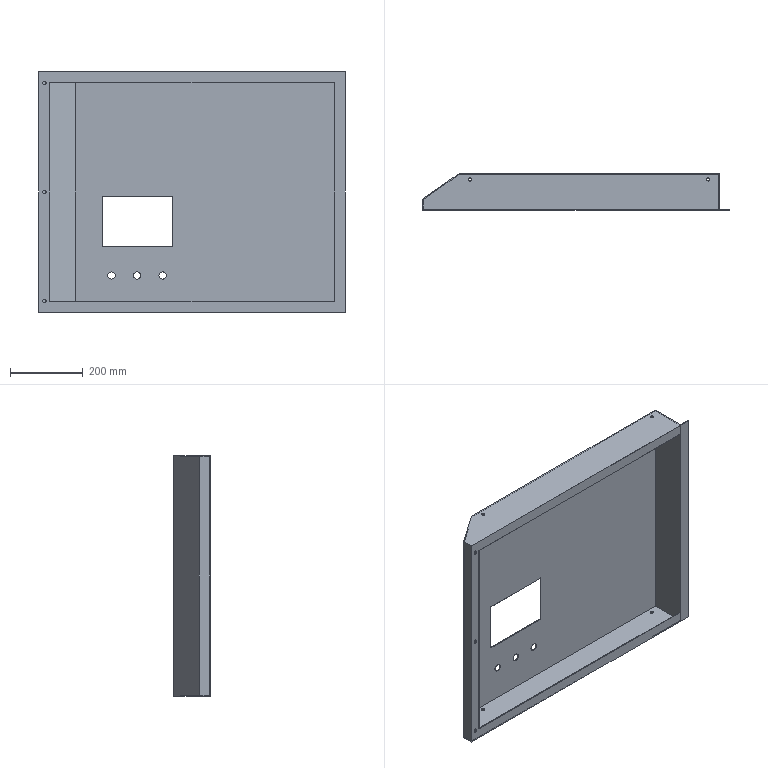Part | SolidWorks | features ICE 5, Extrusion 1, Shell 1 | 1 solid | 43 faces | box 841 x 100 x 658 mm | volume 1673891 mm3 | plane 23 | cylinder 20 | commonest cylinder face diameters 9 x14 20 x6
STEP:
#1=CARTESIAN_POINT('',(-801.5,2.,-299.));
#2=VERTEX_POINT('',#1);
#3=CARTESIAN_POINT('',(-792.5,2.,-299.));
#4=VERTEX_POINT('',#3);
#5=CARTESIAN_POINT('',(-797.,2.,-299.));
#6=DIRECTION('',(0.,-1.,0.));
#7=DIRECTION('',(1.,0.,0.));
#8=AXIS2_PLACEMENT_3D('',#5,#6,#7);
#9=CIRCLE('',#8,4.5);
#10=EDGE_CURVE('',#2,#4,#9,.T.);
#11=ORIENTED_EDGE('',*,*,#10,.F.);
#12=CARTESIAN_POINT('',(-801.5,0.,-299.));
#13=VERTEX_POINT('',#12);
#14=CARTESIAN_POINT('',(-801.5,10.,-299.));
#15=DIRECTION('',(0.,-1.,0.));
#16=VECTOR('',#15,1000.);
#17=LINE('',#14,#16);
#18=EDGE_CURVE('',#2,#13,#17,.T.);
#19=ORIENTED_EDGE('',*,*,#18,.T.);
#20=CARTESIAN_POINT('',(-792.5,0.,-299.));
#21=VERTEX_POINT('',#20);
#22=CARTESIAN_POINT('',(-797.,0.,-299.));
#23=DIRECTION('',(0.,-1.,0.));
#24=DIRECTION('',(1.,0.,0.));
#25=AXIS2_PLACEMENT_3D('',#22,#23,#24);
#26=CIRCLE('',#25,4.5);
#27=EDGE_CURVE('',#13,#21,#26,.T.);
#28=ORIENTED_EDGE('',*,*,#27,.T.);
#29=CARTESIAN_POINT('',(-792.5,10.,-299.));
#30=DIRECTION('',(0.,-1.,0.));
#31=VECTOR('',#30,1000.);
#32=LINE('',#29,#31);
#33=EDGE_CURVE('',#4,#21,#32,.T.);
#34=ORIENTED_EDGE('',*,*,#33,.F.);
#35=EDGE_LOOP('',(#11,#19,#28,#34));
#36=FACE_OUTER_BOUND('',#35,.T.);
#37=CARTESIAN_POINT('',(-797.,10.,-299.));
#38=DIRECTION('',(0.,-1.,0.));
#39=DIRECTION('',(1.,0.,0.));
#40=AXIS2_PLACEMENT_3D('',#37,#38,#39);
#41=CYLINDRICAL_SURFACE('',#40,4.5);
#42=ADVANCED_FACE('',(#36),#41,.F.);
#43=CARTESIAN_POINT('',(-801.5,2.,0.));
#44=VERTEX_POINT('',#43);
#45=CARTESIAN_POINT('',(-792.5,2.,0.));
#46=VERTEX_POINT('',#45);
#47=CARTESIAN_POINT('',(-797.,2.,0.));
#48=DIRECTION('',(0.,-1.,0.));
#49=DIRECTION('',(1.,0.,0.));
#50=AXIS2_PLACEMENT_3D('',#47,#48,#49);
#51=CIRCLE('',#50,4.5);
#52=EDGE_CURVE('',#44,#46,#51,.T.);
#53=ORIENTED_EDGE('',*,*,#52,.F.);
#54=CARTESIAN_POINT('',(-801.5,0.,0.));
#55=VERTEX_POINT('',#54);
#56=CARTESIAN_POINT('',(-801.5,10.,0.));
#57=DIRECTION('',(0.,-1.,0.));
#58=VECTOR('',#57,1000.);
#59=LINE('',#56,#58);
#60=EDGE_CURVE('',#44,#55,#59,.T.);
#61=ORIENTED_EDGE('',*,*,#60,.T.);
#62=CARTESIAN_POINT('',(-792.5,0.,0.));
#63=VERTEX_POINT('',#62);
#64=CARTESIAN_POINT('',(-797.,0.,0.));
#65=DIRECTION('',(0.,-1.,0.));
#66=DIRECTION('',(1.,0.,0.));
#67=AXIS2_PLACEMENT_3D('',#64,#65,#66);
#68=CIRCLE('',#67,4.5);
#69=EDGE_CURVE('',#55,#63,#68,.T.);
#70=ORIENTED_EDGE('',*,*,#69,.T.);
#71=CARTESIAN_POINT('',(-792.5,10.,0.));
#72=DIRECTION('',(0.,-1.,0.));
#73=VECTOR('',#72,1000.);
#74=LINE('',#71,#73);
#75=EDGE_CURVE('',#46,#63,#74,.T.);
#76=ORIENTED_EDGE('',*,*,#75,.F.);
#77=EDGE_LOOP('',(#53,#61,#70,#76));
#78=FACE_OUTER_BOUND('',#77,.T.);
#79=CARTESIAN_POINT('',(-797.,10.,0.));
#80=DIRECTION('',(0.,-1.,0.));
#81=DIRECTION('',(1.,0.,0.));
#82=AXIS2_PLACEMENT_3D('',#79,#80,#81);
#83=CYLINDRICAL_SURFACE('',#82,4.5);
#84=ADVANCED_FACE('',(#78),#83,.F.);
#85=CARTESIAN_POINT('',(-801.5,2.,299.));
#86=VERTEX_POINT('',#85);
#87=CARTESIAN_POINT('',(-792.5,2.,299.));
#88=VERTEX_POINT('',#87);
#89=CARTESIAN_POINT('',(-797.,2.,299.));
#90=DIRECTION('',(0.,-1.,0.));
#91=DIRECTION('',(1.,0.,0.));
#92=AXIS2_PLACEMENT_3D('',#89,#90,#91);
#93=CIRCLE('',#92,4.5);
#94=EDGE_CURVE('',#86,#88,#93,.T.);
#95=ORIENTED_EDGE('',*,*,#94,.F.);
#96=CARTESIAN_POINT('',(-801.5,0.,299.));
#97=VERTEX_POINT('',#96);
#98=CARTESIAN_POINT('',(-801.5,10.,299.));
#99=DIRECTION('',(0.,-1.,0.));
#100=VECTOR('',#99,1000.);
#101=LINE('',#98,#100);
#102=EDGE_CURVE('',#86,#97,#101,.T.);
#103=ORIENTED_EDGE('',*,*,#102,.T.);
#104=CARTESIAN_POINT('',(-792.5,0.,299.));
#105=VERTEX_POINT('',#104);
#106=CARTESIAN_POINT('',(-797.,0.,299.));
#107=DIRECTION('',(0.,-1.,0.));
#108=DIRECTION('',(1.,0.,0.));
#109=AXIS2_PLACEMENT_3D('',#106,#107,#108);
#110=CIRCLE('',#109,4.5);
#111=EDGE_CURVE('',#97,#105,#110,.T.);
#112=ORIENTED_EDGE('',*,*,#111,.T.);
#113=CARTESIAN_POINT('',(-792.5,10.,299.));
#114=DIRECTION('',(0.,-1.,0.));
#115=VECTOR('',#114,1000.);
#116=LINE('',#113,#115);
#117=EDGE_CURVE('',#88,#105,#116,.T.);
#118=ORIENTED_EDGE('',*,*,#117,.F.);
#119=EDGE_LOOP('',(#95,#103,#112,#118));
#120=FACE_OUTER_BOUND('',#119,.T.);
#121=CARTESIAN_POINT('',(-797.,10.,299.));
#122=DIRECTION('',(0.,-1.,0.));
#123=DIRECTION('',(1.,0.,0.));
#124=AXIS2_PLACEMENT_3D('',#121,#122,#123);
#125=CYLINDRICAL_SURFACE('',#124,4.5);
#126=ADVANCED_FACE('',(#120),#125,.F.);
#127=CARTESIAN_POINT('',(-34.5,84.,327.));
#128=VERTEX_POINT('',#127);
#129=CARTESIAN_POINT('',(-25.5,84.,327.));
#130=VERTEX_POINT('',#129);
#131=CARTESIAN_POINT('',(-30.,84.,327.));
#132=DIRECTION('',(0.,0.,1.));
#133=DIRECTION('',(1.,0.,0.));
#134=AXIS2_PLACEMENT_3D('',#131,#132,#133);
#135=CIRCLE('',#134,4.5);
#136=EDGE_CURVE('',#128,#130,#135,.T.);
#137=ORIENTED_EDGE('',*,*,#136,.F.);
#138=CARTESIAN_POINT('',(-34.5,84.,329.));
#139=VERTEX_POINT('',#138);
#140=CARTESIAN_POINT('',(-34.5,84.,-468.));
#141=DIRECTION('',(0.,0.,1.));
#142=VECTOR('',#141,1000.);
#143=LINE('',#140,#142);
#144=EDGE_CURVE('',#128,#139,#143,.T.);
#145=ORIENTED_EDGE('',*,*,#144,.T.);
#146=CARTESIAN_POINT('',(-25.5,84.,329.));
#147=VERTEX_POINT('',#146);
#148=CARTESIAN_POINT('',(-30.,84.,329.));
#149=DIRECTION('',(0.,0.,1.));
#150=DIRECTION('',(1.,0.,0.));
#151=AXIS2_PLACEMENT_3D('',#148,#149,#150);
#152=CIRCLE('',#151,4.5);
#153=EDGE_CURVE('',#139,#147,#152,.T.);
#154=ORIENTED_EDGE('',*,*,#153,.T.);
#155=CARTESIAN_POINT('',(-25.5,84.,-468.));
#156=DIRECTION('',(0.,0.,1.));
#157=VECTOR('',#156,1000.);
#158=LINE('',#155,#157);
#159=EDGE_CURVE('',#130,#147,#158,.T.);
#160=ORIENTED_EDGE('',*,*,#159,.F.);
#161=EDGE_LOOP('',(#137,#145,#154,#160));
#162=FACE_OUTER_BOUND('',#161,.T.);
#163=CARTESIAN_POINT('',(-30.,84.,-468.));
#164=DIRECTION('',(0.,0.,1.));
#165=DIRECTION('',(1.,0.,0.));
#166=AXIS2_PLACEMENT_3D('',#163,#164,#165);
#167=CYLINDRICAL_SURFACE('',#166,4.5);
#168=ADVANCED_FACE('',(#162),#167,.F.);
#169=CARTESIAN_POINT('',(-34.5,84.,-329.));
#170=VERTEX_POINT('',#169);
#171=CARTESIAN_POINT('',(-25.5,84.,-329.));
#172=VERTEX_POINT('',#171);
#173=CARTESIAN_POINT('',(-30.,84.,-329.));
#174=DIRECTION('',(0.,0.,1.));
#175=DIRECTION('',(1.,0.,0.));
#176=AXIS2_PLACEMENT_3D('',#173,#174,#175);
#177=CIRCLE('',#176,4.5);
#178=EDGE_CURVE('',#170,#172,#177,.T.);
#179=ORIENTED_EDGE('',*,*,#178,.F.);
#180=CARTESIAN_POINT('',(-34.5,84.,-327.));
#181=VERTEX_POINT('',#180);
#182=CARTESIAN_POINT('',(-34.5,84.,-468.));
#183=DIRECTION('',(0.,0.,1.));
#184=VECTOR('',#183,1000.);
#185=LINE('',#182,#184);
#186=EDGE_CURVE('',#170,#181,#185,.T.);
#187=ORIENTED_EDGE('',*,*,#186,.T.);
#188=CARTESIAN_POINT('',(-25.5,84.,-327.));
#189=VERTEX_POINT('',#188);
#190=CARTESIAN_POINT('',(-30.,84.,-327.));
#191=DIRECTION('',(0.,0.,1.));
#192=DIRECTION('',(1.,0.,0.));
#193=AXIS2_PLACEMENT_3D('',#190,#191,#192);
#194=CIRCLE('',#193,4.5);
#195=EDGE_CURVE('',#181,#189,#194,.T.);
#196=ORIENTED_EDGE('',*,*,#195,.T.);
#197=CARTESIAN_POINT('',(-25.5,84.,-468.));
#198=DIRECTION('',(0.,0.,1.));
#199=VECTOR('',#198,1000.);
#200=LINE('',#197,#199);
#201=EDGE_CURVE('',#172,#189,#200,.T.);
#202=ORIENTED_EDGE('',*,*,#201,.F.);
#203=EDGE_LOOP('',(#179,#187,#196,#202));
#204=FACE_OUTER_BOUND('',#203,.T.);
#205=CARTESIAN_POINT('',(-30.,84.,-468.));
#206=DIRECTION('',(0.,0.,1.));
#207=DIRECTION('',(1.,0.,0.));
#208=AXIS2_PLACEMENT_3D('',#205,#206,#207);
#209=CYLINDRICAL_SURFACE('',#208,4.5);
#210=ADVANCED_FACE('',(#204),#209,.F.);
#211=CARTESIAN_POINT('',(-687.53,84.,327.));
#212=VERTEX_POINT('',#211);
#213=CARTESIAN_POINT('',(-678.53,84.,327.));
#214=VERTEX_POINT('',#213);
#215=CARTESIAN_POINT('',(-683.03,84.,327.));
#216=DIRECTION('',(0.,0.,1.));
#217=DIRECTION('',(1.,0.,0.));
#218=AXIS2_PLACEMENT_3D('',#215,#216,#217);
#219=CIRCLE('',#218,4.5);
#220=EDGE_CURVE('',#212,#214,#219,.T.);
#221=ORIENTED_EDGE('',*,*,#220,.F.);
#222=CARTESIAN_POINT('',(-687.53,84.,329.));
#223=VERTEX_POINT('',#222);
#224=CARTESIAN_POINT('',(-687.53,84.,-468.));
#225=DIRECTION('',(0.,0.,1.));
#226=VECTOR('',#225,1000.);
#227=LINE('',#224,#226);
#228=EDGE_CURVE('',#212,#223,#227,.T.);
#229=ORIENTED_EDGE('',*,*,#228,.T.);
#230=CARTESIAN_POINT('',(-678.53,84.,329.));
#231=VERTEX_POINT('',#230);
#232=CARTESIAN_POINT('',(-683.03,84.,329.));
#233=DIRECTION('',(0.,0.,1.));
#234=DIRECTION('',(1.,0.,0.));
#235=AXIS2_PLACEMENT_3D('',#232,#233,#234);
#236=CIRCLE('',#235,4.5);
#237=EDGE_CURVE('',#223,#231,#236,.T.);
#238=ORIENTED_EDGE('',*,*,#237,.T.);
#239=CARTESIAN_POINT('',(-678.53,84.,-468.));
#240=DIRECTION('',(0.,0.,1.));
#241=VECTOR('',#240,1000.);
#242=LINE('',#239,#241);
#243=EDGE_CURVE('',#214,#231,#242,.T.);
#244=ORIENTED_EDGE('',*,*,#243,.F.);
#245=EDGE_LOOP('',(#221,#229,#238,#244));
#246=FACE_OUTER_BOUND('',#245,.T.);
#247=CARTESIAN_POINT('',(-683.03,84.,-468.));
#248=DIRECTION('',(0.,0.,1.));
#249=DIRECTION('',(1.,0.,0.));
#250=AXIS2_PLACEMENT_3D('',#247,#248,#249);
#251=CYLINDRICAL_SURFACE('',#250,4.5);
#252=ADVANCED_FACE('',(#246),#251,.F.);
#253=CARTESIAN_POINT('',(-687.53,84.,-329.));
#254=VERTEX_POINT('',#253);
#255=CARTESIAN_POINT('',(-678.53,84.,-329.));
#256=VERTEX_POINT('',#255);
#257=CARTESIAN_POINT('',(-683.03,84.,-329.));
#258=DIRECTION('',(0.,0.,1.));
#259=DIRECTION('',(1.,0.,0.));
#260=AXIS2_PLACEMENT_3D('',#257,#258,#259);
#261=CIRCLE('',#260,4.5);
#262=EDGE_CURVE('',#254,#256,#261,.T.);
#263=ORIENTED_EDGE('',*,*,#262,.F.);
#264=CARTESIAN_POINT('',(-687.53,84.,-327.));
#265=VERTEX_POINT('',#264);
#266=CARTESIAN_POINT('',(-687.53,84.,-468.));
#267=DIRECTION('',(0.,0.,1.));
#268=VECTOR('',#267,1000.);
#269=LINE('',#266,#268);
#270=EDGE_CURVE('',#254,#265,#269,.T.);
#271=ORIENTED_EDGE('',*,*,#270,.T.);
#272=CARTESIAN_POINT('',(-678.53,84.,-327.));
#273=VERTEX_POINT('',#272);
#274=CARTESIAN_POINT('',(-683.03,84.,-327.));
#275=DIRECTION('',(0.,0.,1.));
#276=DIRECTION('',(1.,0.,0.));
#277=AXIS2_PLACEMENT_3D('',#274,#275,#276);
#278=CIRCLE('',#277,4.5);
#279=EDGE_CURVE('',#265,#273,#278,.T.);
#280=ORIENTED_EDGE('',*,*,#279,.T.);
#281=CARTESIAN_POINT('',(-678.53,84.,-468.));
#282=DIRECTION('',(0.,0.,1.));
#283=VECTOR('',#282,1000.);
#284=LINE('',#281,#283);
#285=EDGE_CURVE('',#256,#273,#284,.T.);
#286=ORIENTED_EDGE('',*,*,#285,.F.);
#287=EDGE_LOOP('',(#263,#271,#280,#286));
#288=FACE_OUTER_BOUND('',#287,.T.);
#289=CARTESIAN_POINT('',(-683.03,84.,-468.));
#290=DIRECTION('',(0.,0.,1.));
#291=DIRECTION('',(1.,0.,0.));
#292=AXIS2_PLACEMENT_3D('',#289,#290,#291);
#293=CYLINDRICAL_SURFACE('',#292,4.5);
#294=ADVANCED_FACE('',(#288),#293,.F.);
#295=CARTESIAN_POINT('',(-483.03,98.,-229.));
#296=VERTEX_POINT('',#295);
#297=CARTESIAN_POINT('',(-463.03,98.,-229.));
#298=VERTEX_POINT('',#297);
#299=CARTESIAN_POINT('',(-473.03,98.,-229.));
#300=DIRECTION('',(0.,-1.,0.));
#301=DIRECTION('',(1.,0.,0.));
#302=AXIS2_PLACEMENT_3D('',#299,#300,#301);
#303=CIRCLE('',#302,10.);
#304=EDGE_CURVE('',#296,#298,#303,.T.);
#305=ORIENTED_EDGE('',*,*,#304,.T.);
#306=CARTESIAN_POINT('',(-463.03,100.,-229.));
#307=VERTEX_POINT('',#306);
#308=CARTESIAN_POINT('',(-463.03,-558.,-229.));
#309=DIRECTION('',(0.,1.,0.));
#310=VECTOR('',#309,1000.);
#311=LINE('',#308,#310);
#312=EDGE_CURVE('',#298,#307,#311,.T.);
#313=ORIENTED_EDGE('',*,*,#312,.T.);
#314=CARTESIAN_POINT('',(-483.03,100.,-229.));
#315=VERTEX_POINT('',#314);
#316=CARTESIAN_POINT('',(-473.03,100.,-229.));
#317=DIRECTION('',(0.,1.,0.));
#318=DIRECTION('',(1.,0.,0.));
#319=AXIS2_PLACEMENT_3D('',#316,#317,#318);
#320=CIRCLE('',#319,10.);
#321=EDGE_CURVE('',#307,#315,#320,.T.);
#322=ORIENTED_EDGE('',*,*,#321,.T.);
#323=CARTESIAN_POINT('',(-483.03,-558.,-229.));
#324=DIRECTION('',(0.,1.,0.));
#325=VECTOR('',#324,1000.);
#326=LINE('',#323,#325);
#327=EDGE_CURVE('',#296,#315,#326,.T.);
#328=ORIENTED_EDGE('',*,*,#327,.F.);
#329=EDGE_LOOP('',(#305,#313,#322,#328));
#330=FACE_OUTER_BOUND('',#329,.T.);
#331=CARTESIAN_POINT('',(-473.03,-558.,-229.));
#332=DIRECTION('',(0.,1.,0.));
#333=DIRECTION('',(-1.,0.,0.));
#334=AXIS2_PLACEMENT_3D('',#331,#332,#333);
#335=CYLINDRICAL_SURFACE('',#334,10.);
#336=ADVANCED_FACE('',(#330),#335,.F.);
#337=CARTESIAN_POINT('',(-553.03,98.,-229.));
#338=VERTEX_POINT('',#337);
#339=CARTESIAN_POINT('',(-533.03,98.,-229.));
#340=VERTEX_POINT('',#339);
#341=CARTESIAN_POINT('',(-543.03,98.,-229.));
#342=DIRECTION('',(0.,-1.,0.));
#343=DIRECTION('',(1.,0.,0.));
#344=AXIS2_PLACEMENT_3D('',#341,#342,#343);
#345=CIRCLE('',#344,10.);
#346=EDGE_CURVE('',#338,#340,#345,.T.);
#347=ORIENTED_EDGE('',*,*,#346,.T.);
#348=CARTESIAN_POINT('',(-533.03,100.,-229.));
#349=VERTEX_POINT('',#348);
#350=CARTESIAN_POINT('',(-533.03,-558.,-229.));
#351=DIRECTION('',(0.,1.,0.));
#352=VECTOR('',#351,1000.);
#353=LINE('',#350,#352);
#354=EDGE_CURVE('',#340,#349,#353,.T.);
#355=ORIENTED_EDGE('',*,*,#354,.T.);
#356=CARTESIAN_POINT('',(-553.03,100.,-229.));
#357=VERTEX_POINT('',#356);
#358=CARTESIAN_POINT('',(-543.03,100.,-229.));
#359=DIRECTION('',(0.,1.,0.));
#360=DIRECTION('',(-1.,0.,0.));
#361=AXIS2_PLACEMENT_3D('',#358,#359,#360);
#362=CIRCLE('',#361,10.);
#363=EDGE_CURVE('',#349,#357,#362,.T.);
#364=ORIENTED_EDGE('',*,*,#363,.T.);
#365=CARTESIAN_POINT('',(-553.03,-558.,-229.));
#366=DIRECTION('',(0.,1.,0.));
#367=VECTOR('',#366,1000.);
#368=LINE('',#365,#367);
#369=EDGE_CURVE('',#338,#357,#368,.T.);
#370=ORIENTED_EDGE('',*,*,#369,.F.);
#371=EDGE_LOOP('',(#347,#355,#364,#370));
#372=FACE_OUTER_BOUND('',#371,.T.);
#373=CARTESIAN_POINT('',(-543.03,-558.,-229.));
#374=DIRECTION('',(0.,1.,0.));
#375=DIRECTION('',(-1.,0.,0.));
#376=AXIS2_PLACEMENT_3D('',#373,#374,#375);
#377=CYLINDRICAL_SURFACE('',#376,10.);
#378=ADVANCED_FACE('',(#372),#377,.F.);
#379=CARTESIAN_POINT('',(-623.03,98.,-229.));
#380=VERTEX_POINT('',#379);
#381=CARTESIAN_POINT('',(-603.03,98.,-229.));
#382=VERTEX_POINT('',#381);
#383=CARTESIAN_POINT('',(-613.03,98.,-229.));
#384=DIRECTION('',(0.,-1.,0.));
#385=DIRECTION('',(1.,0.,0.));
#386=AXIS2_PLACEMENT_3D('',#383,#384,#385);
#387=CIRCLE('',#386,10.);
#388=EDGE_CURVE('',#380,#382,#387,.T.);
#389=ORIENTED_EDGE('',*,*,#388,.T.);
#390=CARTESIAN_POINT('',(-603.03,100.,-229.));
#391=VERTEX_POINT('',#390);
#392=CARTESIAN_POINT('',(-603.03,-558.,-229.));
#393=DIRECTION('',(0.,1.,0.));
#394=VECTOR('',#393,1000.);
#395=LINE('',#392,#394);
#396=EDGE_CURVE('',#382,#391,#395,.T.);
#397=ORIENTED_EDGE('',*,*,#396,.T.);
#398=CARTESIAN_POINT('',(-623.03,100.,-229.));
#399=VERTEX_POINT('',#398);
#400=CARTESIAN_POINT('',(-613.03,100.,-229.));
#401=DIRECTION('',(0.,1.,0.));
#402=DIRECTION('',(-1.,0.,0.));
#403=AXIS2_PLACEMENT_3D('',#400,#401,#402);
#404=CIRCLE('',#403,10.);
#405=EDGE_CURVE('',#391,#399,#404,.T.);
#406=ORIENTED_EDGE('',*,*,#405,.T.);
#407=CARTESIAN_POINT('',(-623.03,-558.,-229.));
#408=DIRECTION('',(0.,1.,0.));
#409=VECTOR('',#408,1000.);
#410=LINE('',#407,#409);
#411=EDGE_CURVE('',#380,#399,#410,.T.);
#412=ORIENTED_EDGE('',*,*,#411,.F.);
#413=EDGE_LOOP('',(#389,#397,#406,#412));
#414=FACE_OUTER_BOUND('',#413,.T.);
#415=CARTESIAN_POINT('',(-613.03,-558.,-229.));
#416=DIRECTION('',(0.,1.,0.));
#417=DIRECTION('',(-1.,0.,0.));
#418=AXIS2_PLACEMENT_3D('',#415,#416,#417);
#419=CYLINDRICAL_SURFACE('',#418,10.);
#420=ADVANCED_FACE('',(#414),#419,.F.);
#421=CARTESIAN_POINT('',(-811.,28.959,327.));
#422=VERTEX_POINT('',#421);
#423=CARTESIAN_POINT('',(-811.,2.,327.));
#424=VERTEX_POINT('',#423);
#425=CARTESIAN_POINT('',(-811.,0.,327.));
#426=DIRECTION('',(0.,-1.,0.));
#427=VECTOR('',#426,1000.);
#428=LINE('',#425,#427);
#429=EDGE_CURVE('',#422,#424,#428,.T.);
#430=ORIENTED_EDGE('',*,*,#429,.T.);
#431=CARTESIAN_POINT('',(-811.,2.,-327.));
#432=VERTEX_POINT('',#431);
#433=CARTESIAN_POINT('',(-811.,2.,329.));
#434=DIRECTION('',(0.,0.,-1.));
#435=VECTOR('',#434,1000.);
#436=LINE('',#433,#435);
#437=EDGE_CURVE('',#424,#432,#436,.T.);
#438=ORIENTED_EDGE('',*,*,#437,.T.);
#439=CARTESIAN_POINT('',(-811.,28.959,-327.));
#440=VERTEX_POINT('',#439);
#441=CARTESIAN_POINT('',(-811.,0.,-327.));
#442=DIRECTION('',(0.,-1.,0.));
#443=VECTOR('',#442,1000.);
#444=LINE('',#441,#443);
#445=EDGE_CURVE('',#440,#432,#444,.T.);
#446=ORIENTED_EDGE('',*,*,#445,.F.);
#447=CARTESIAN_POINT('',(-811.,28.959,329.));
#448=DIRECTION('',(0.,0.,-1.));
#449=VECTOR('',#448,1000.);
#450=LINE('',#447,#449);
#451=EDGE_CURVE('',#422,#440,#450,.T.);
#452=ORIENTED_EDGE('',*,*,#451,.F.);
#453=EDGE_LOOP('',(#430,#438,#446,#452));
#454=FACE_OUTER_BOUND('',#453,.T.);
#455=CARTESIAN_POINT('',(-811.,0.,329.));
#456=DIRECTION('',(1.,0.,0.));
#457=DIRECTION('',(0.,1.,0.));
#458=AXIS2_PLACEMENT_3D('',#455,#456,#457);
#459=PLANE('',#458);
#460=ADVANCED_FACE('',(#454),#459,.T.);
#461=CARTESIAN_POINT('',(-30.,84.,327.));
#462=DIRECTION('',(0.,0.,1.));
#463=DIRECTION('',(1.,0.,0.));
#464=AXIS2_PLACEMENT_3D('',#461,#462,#463);
#465=CIRCLE('',#464,4.5);
#466=EDGE_CURVE('',#130,#128,#465,.T.);
#467=ORIENTED_EDGE('',*,*,#466,.T.);
#468=ORIENTED_EDGE('',*,*,#136,.T.);
#469=EDGE_LOOP('',(#467,#468));
#470=FACE_BOUND('',#469,.T.);
#471=CARTESIAN_POINT('',(-683.03,84.,327.));
#472=DIRECTION('',(0.,0.,1.));
#473=DIRECTION('',(1.,0.,0.));
#474=AXIS2_PLACEMENT_3D('',#471,#472,#473);
#475=CIRCLE('',#474,4.5);
#476=EDGE_CURVE('',#214,#212,#475,.T.);
#477=ORIENTED_EDGE('',*,*,#476,.T.);
#478=ORIENTED_EDGE('',*,*,#220,.T.);
#479=EDGE_LOOP('',(#477,#478));
#480=FACE_BOUND('',#479,.T.);
#481=CARTESIAN_POINT('',(-2.,2.,327.));
#482=VERTEX_POINT('',#481);
#483=CARTESIAN_POINT('',(0.,2.,327.));
#484=DIRECTION('',(1.,0.,0.));
#485=VECTOR('',#484,1000.);
#486=LINE('',#483,#485);
#487=EDGE_CURVE('',#424,#482,#486,.T.);
#488=ORIENTED_EDGE('',*,*,#487,.F.);
#489=ORIENTED_EDGE('',*,*,#429,.F.);
#490=CARTESIAN_POINT('',(-712.399,98.,327.));
#491=VERTEX_POINT('',#490);
#492=CARTESIAN_POINT('',(-711.882,98.362,327.));
#493=DIRECTION('',(-0.8192,-0.5736,0.));
#494=VECTOR('',#493,1000.);
#495=LINE('',#492,#494);
#496=EDGE_CURVE('',#491,#422,#495,.T.);
#497=ORIENTED_EDGE('',*,*,#496,.F.);
#498=CARTESIAN_POINT('',(-2.,98.,327.));
#499=VERTEX_POINT('',#498);
#500=CARTESIAN_POINT('',(0.,98.,327.));
#501=DIRECTION('',(-1.,0.,0.));
#502=VECTOR('',#501,1000.);
#503=LINE('',#500,#502);
#504=EDGE_CURVE('',#499,#491,#503,.T.);
#505=ORIENTED_EDGE('',*,*,#504,.F.);
#506=CARTESIAN_POINT('',(-2.,0.,327.));
#507=DIRECTION('',(0.,1.,0.));
#508=VECTOR('',#507,1000.);
#509=LINE('',#506,#508);
#510=EDGE_CURVE('',#482,#499,#509,.T.);
#511=ORIENTED_EDGE('',*,*,#510,.F.);
#512=EDGE_LOOP('',(#488,#489,#497,#505,#511));
#513=FACE_OUTER_BOUND('',#512,.T.);
#514=CARTESIAN_POINT('',(0.,100.,327.));
#515=DIRECTION('',(0.,0.,1.));
#516=DIRECTION('',(1.,0.,0.));
#517=AXIS2_PLACEMENT_3D('',#514,#515,#516);
#518=PLANE('',#517);
#519=ADVANCED_FACE('',(#470,#480,#513),#518,.F.);
#520=CARTESIAN_POINT('',(-30.,84.,-327.));
#521=DIRECTION('',(0.,0.,1.));
#522=DIRECTION('',(1.,0.,0.));
#523=AXIS2_PLACEMENT_3D('',#520,#521,#522);
#524=CIRCLE('',#523,4.5);
#525=EDGE_CURVE('',#189,#181,#524,.T.);
#526=ORIENTED_EDGE('',*,*,#525,.F.);
#527=ORIENTED_EDGE('',*,*,#195,.F.);
#528=EDGE_LOOP('',(#526,#527));
#529=FACE_BOUND('',#528,.T.);
#530=CARTESIAN_POINT('',(-683.03,84.,-327.));
#531=DIRECTION('',(0.,0.,1.));
#532=DIRECTION('',(1.,0.,0.));
#533=AXIS2_PLACEMENT_3D('',#530,#531,#532);
#534=CIRCLE('',#533,4.5);
#535=EDGE_CURVE('',#273,#265,#534,.T.);
#536=ORIENTED_EDGE('',*,*,#535,.F.);
#537=ORIENTED_EDGE('',*,*,#279,.F.);
#538=EDGE_LOOP('',(#536,#537));
#539=FACE_BOUND('',#538,.T.);
#540=ORIENTED_EDGE('',*,*,#445,.T.);
#541=CARTESIAN_POINT('',(-2.,2.,-327.));
#542=VERTEX_POINT('',#541);
#543=CARTESIAN_POINT('',(0.,2.,-327.));
#544=DIRECTION('',(1.,0.,0.));
#545=VECTOR('',#544,1000.);
#546=LINE('',#543,#545);
#547=EDGE_CURVE('',#432,#542,#546,.T.);
#548=ORIENTED_EDGE('',*,*,#547,.T.);
#549=CARTESIAN_POINT('',(-2.,98.,-327.));
#550=VERTEX_POINT('',#549);
#551=CARTESIAN_POINT('',(-2.,0.,-327.));
#552=DIRECTION('',(0.,1.,0.));
#553=VECTOR('',#552,1000.);
#554=LINE('',#551,#553);
#555=EDGE_CURVE('',#542,#550,#554,.T.);
#556=ORIENTED_EDGE('',*,*,#555,.T.);
#557=CARTESIAN_POINT('',(-712.399,98.,-327.));
#558=VERTEX_POINT('',#557);
#559=CARTESIAN_POINT('',(0.,98.,-327.));
#560=DIRECTION('',(-1.,0.,0.));
#561=VECTOR('',#560,1000.);
#562=LINE('',#559,#561);
#563=EDGE_CURVE('',#550,#558,#562,.T.);
#564=ORIENTED_EDGE('',*,*,#563,.T.);
#565=CARTESIAN_POINT('',(-711.882,98.362,-327.));
#566=DIRECTION('',(-0.8192,-0.5736,0.));
#567=VECTOR('',#566,1000.);
#568=LINE('',#565,#567);
#569=EDGE_CURVE('',#558,#440,#568,.T.);
#570=ORIENTED_EDGE('',*,*,#569,.T.);
#571=EDGE_LOOP('',(#540,#548,#556,#564,#570));
#572=FACE_OUTER_BOUND('',#571,.T.);
#573=CARTESIAN_POINT('',(0.,100.,-327.));
#574=DIRECTION('',(0.,0.,1.));
#575=DIRECTION('',(1.,0.,0.));
#576=AXIS2_PLACEMENT_3D('',#573,#574,#575);
#577=PLANE('',#576);
#578=ADVANCED_FACE('',(#529,#539,#572),#577,.T.);
#579=CARTESIAN_POINT('',(0.,2.,-329.));
#580=VERTEX_POINT('',#579);
#581=CARTESIAN_POINT('',(0.,2.,329.));
#582=VERTEX_POINT('',#581);
#583=CARTESIAN_POINT('',(0.,2.,329.));
#584=DIRECTION('',(0.,0.,1.));
#585=VECTOR('',#584,1000.);
#586=LINE('',#583,#585);
#587=EDGE_CURVE('',#580,#582,#586,.T.);
#588=ORIENTED_EDGE('',*,*,#587,.F.);
#589=CARTESIAN_POINT('',(0.,100.,-329.));
#590=VERTEX_POINT('',#589);
#591=CARTESIAN_POINT('',(0.,0.,-329.));
#592=DIRECTION('',(0.,1.,0.));
#593=VECTOR('',#592,1000.);
#594=LINE('',#591,#593);
#595=EDGE_CURVE('',#580,#590,#594,.T.);
#596=ORIENTED_EDGE('',*,*,#595,.T.);
#597=CARTESIAN_POINT('',(0.,100.,329.));
#598=VERTEX_POINT('',#597);
#599=CARTESIAN_POINT('',(0.,100.,329.));
#600=DIRECTION('',(0.,0.,-1.));
#601=VECTOR('',#600,1000.);
#602=LINE('',#599,#601);
#603=EDGE_CURVE('',#598,#590,#602,.T.);
#604=ORIENTED_EDGE('',*,*,#603,.F.);
#605=CARTESIAN_POINT('',(0.,0.,329.));
#606=DIRECTION('',(0.,1.,0.));
#607=VECTOR('',#606,1000.);
#608=LINE('',#605,#607);
#609=EDGE_CURVE('',#582,#598,#608,.T.);
#610=ORIENTED_EDGE('',*,*,#609,.F.);
#611=EDGE_LOOP('',(#588,#596,#604,#610));
#612=FACE_OUTER_BOUND('',#611,.T.);
#613=CARTESIAN_POINT('',(0.,0.,329.));
#614=DIRECTION('',(-1.,0.,0.));
#615=DIRECTION('',(0.,0.,1.));
#616=AXIS2_PLACEMENT_3D('',#613,#614,#615);
#617=PLANE('',#616);
#618=ADVANCED_FACE('',(#612),#617,.F.);
#619=CARTESIAN_POINT('',(-797.,0.,-299.));
#620=DIRECTION('',(0.,-1.,0.));
#621=DIRECTION('',(1.,0.,0.));
#622=AXIS2_PLACEMENT_3D('',#619,#620,#621);
#623=CIRCLE('',#622,4.5);
#624=EDGE_CURVE('',#21,#13,#623,.T.);
#625=ORIENTED_EDGE('',*,*,#624,.F.);
#626=ORIENTED_EDGE('',*,*,#27,.F.);
#627=EDGE_LOOP('',(#625,#626));
#628=FACE_BOUND('',#627,.T.);
#629=CARTESIAN_POINT('',(-797.,0.,0.));
#630=DIRECTION('',(0.,-1.,0.));
#631=DIRECTION('',(1.,0.,0.));
#632=AXIS2_PLACEMENT_3D('',#629,#630,#631);
#633=CIRCLE('',#632,4.5);
#634=EDGE_CURVE('',#63,#55,#633,.T.);
#635=ORIENTED_EDGE('',*,*,#634,.F.);
#636=ORIENTED_EDGE('',*,*,#69,.F.);
#637=EDGE_LOOP('',(#635,#636));
#638=FACE_BOUND('',#637,.T.);
#639=CARTESIAN_POINT('',(-797.,0.,299.));
#640=DIRECTION('',(0.,-1.,0.));
#641=DIRECTION('',(1.,0.,0.));
#642=AXIS2_PLACEMENT_3D('',#639,#640,#641);
#643=CIRCLE('',#642,4.5);
#644=EDGE_CURVE('',#105,#97,#643,.T.);
#645=ORIENTED_EDGE('',*,*,#644,.F.);
#646=ORIENTED_EDGE('',*,*,#111,.F.);
#647=EDGE_LOOP('',(#645,#646));
#648=FACE_BOUND('',#647,.T.);
#649=CARTESIAN_POINT('',(-783.,0.,299.));
#650=VERTEX_POINT('',#649);
#651=CARTESIAN_POINT('',(-2.,0.,299.));
#652=VERTEX_POINT('',#651);
#653=CARTESIAN_POINT('',(-783.,0.,299.));
#654=DIRECTION('',(1.,0.,0.));
#655=VECTOR('',#654,1000.);
#656=LINE('',#653,#655);
#657=EDGE_CURVE('',#650,#652,#656,.T.);
#658=ORIENTED_EDGE('',*,*,#657,.T.);
#659=CARTESIAN_POINT('',(-2.,0.,-299.));
#660=VERTEX_POINT('',#659);
#661=CARTESIAN_POINT('',(-2.,0.,329.));
#662=DIRECTION('',(0.,0.,-1.));
#663=VECTOR('',#662,1000.);
#664=LINE('',#661,#663);
#665=EDGE_CURVE('',#652,#660,#664,.T.);
#666=ORIENTED_EDGE('',*,*,#665,.T.);
#667=CARTESIAN_POINT('',(-783.,0.,-299.));
#668=VERTEX_POINT('',#667);
#669=CARTESIAN_POINT('',(-783.,0.,-299.));
#670=DIRECTION('',(-1.,0.,0.));
#671=VECTOR('',#670,1000.);
#672=LINE('',#669,#671);
#673=EDGE_CURVE('',#660,#668,#672,.T.);
#674=ORIENTED_EDGE('',*,*,#673,.T.);
#675=CARTESIAN_POINT('',(-783.,0.,299.));
#676=DIRECTION('',(0.,0.,1.));
#677=VECTOR('',#676,1000.);
#678=LINE('',#675,#677);
#679=EDGE_CURVE('',#668,#650,#678,.T.);
#680=ORIENTED_EDGE('',*,*,#679,.T.);
#681=EDGE_LOOP('',(#658,#666,#674,#680));
#682=FACE_BOUND('',#681,.T.);
#683=CARTESIAN_POINT('',(28.,0.,-329.));
#684=VERTEX_POINT('',#683);
#685=CARTESIAN_POINT('',(28.,0.,329.));
#686=VERTEX_POINT('',#685);
#687=CARTESIAN_POINT('',(28.,0.,329.));
#688=DIRECTION('',(0.,0.,1.));
#689=VECTOR('',#688,1000.);
#690=LINE('',#687,#689);
#691=EDGE_CURVE('',#684,#686,#690,.T.);
#692=ORIENTED_EDGE('',*,*,#691,.T.);
#693=CARTESIAN_POINT('',(-813.,0.,329.));
#694=VERTEX_POINT('',#693);
#695=CARTESIAN_POINT('',(0.,0.,329.));
#696=DIRECTION('',(1.,0.,0.));
#697=VECTOR('',#696,1000.);
#698=LINE('',#695,#697);
#699=EDGE_CURVE('',#694,#686,#698,.T.);
#700=ORIENTED_EDGE('',*,*,#699,.F.);
#701=CARTESIAN_POINT('',(-813.,0.,-329.));
#702=VERTEX_POINT('',#701);
#703=CARTESIAN_POINT('',(-813.,0.,329.));
#704=DIRECTION('',(0.,0.,-1.));
#705=VECTOR('',#704,1000.);
#706=LINE('',#703,#705);
#707=EDGE_CURVE('',#694,#702,#706,.T.);
#708=ORIENTED_EDGE('',*,*,#707,.T.);
#709=CARTESIAN_POINT('',(0.,0.,-329.));
#710=DIRECTION('',(1.,0.,0.));
#711=VECTOR('',#710,1000.);
#712=LINE('',#709,#711);
#713=EDGE_CURVE('',#702,#684,#712,.T.);
#714=ORIENTED_EDGE('',*,*,#713,.T.);
#715=EDGE_LOOP('',(#692,#700,#708,#714));
#716=FACE_OUTER_BOUND('',#715,.T.);
#717=CARTESIAN_POINT('',(0.,0.,329.));
#718=DIRECTION('',(0.,1.,0.));
#719=DIRECTION('',(-1.,0.,0.));
#720=AXIS2_PLACEMENT_3D('',#717,#718,#719);
#721=PLANE('',#720);
#722=ADVANCED_FACE('',(#628,#638,#648,#682,#716),#721,.F.);
#723=CARTESIAN_POINT('',(-473.03,100.,-229.));
#724=DIRECTION('',(0.,1.,0.));
#725=DIRECTION('',(1.,0.,0.));
#726=AXIS2_PLACEMENT_3D('',#723,#724,#725);
#727=CIRCLE('',#726,10.);
#728=EDGE_CURVE('',#315,#307,#727,.T.);
#729=ORIENTED_EDGE('',*,*,#728,.F.);
#730=ORIENTED_EDGE('',*,*,#321,.F.);
#731=EDGE_LOOP('',(#729,#730));
#732=FACE_BOUND('',#731,.T.);
#733=CARTESIAN_POINT('',(-543.03,100.,-229.));
#734=DIRECTION('',(0.,1.,0.));
#735=DIRECTION('',(-1.,0.,0.));
#736=AXIS2_PLACEMENT_3D('',#733,#734,#735);
#737=CIRCLE('',#736,10.);
#738=EDGE_CURVE('',#357,#349,#737,.T.);
#739=ORIENTED_EDGE('',*,*,#738,.F.);
#740=ORIENTED_EDGE('',*,*,#363,.F.);
#741=EDGE_LOOP('',(#739,#740));
#742=FACE_BOUND('',#741,.T.);
#743=CARTESIAN_POINT('',(-613.03,100.,-229.));
#744=DIRECTION('',(0.,1.,0.));
#745=DIRECTION('',(-1.,0.,0.));
#746=AXIS2_PLACEMENT_3D('',#743,#744,#745);
#747=CIRCLE('',#746,10.);
#748=EDGE_CURVE('',#399,#391,#747,.T.);
#749=ORIENTED_EDGE('',*,*,#748,.F.);
#750=ORIENTED_EDGE('',*,*,#405,.F.);
#751=EDGE_LOOP('',(#749,#750));
#752=FACE_BOUND('',#751,.T.);
#753=CARTESIAN_POINT('',(-639.03,100.,-11.));
#754=VERTEX_POINT('',#753);
#755=CARTESIAN_POINT('',(-447.03,100.,-11.));
#756=VERTEX_POINT('',#755);
#757=CARTESIAN_POINT('',(-639.03,100.,-11.));
#758=DIRECTION('',(1.,0.,0.));
#759=VECTOR('',#758,1000.);
#760=LINE('',#757,#759);
#761=EDGE_CURVE('',#754,#756,#760,.T.);
#762=ORIENTED_EDGE('',*,*,#761,.F.);
#763=CARTESIAN_POINT('',(-639.03,100.,-149.));
#764=VERTEX_POINT('',#763);
#765=CARTESIAN_POINT('',(-639.03,100.,-149.));
#766=DIRECTION('',(0.,0.,1.));
#767=VECTOR('',#766,1000.);
#768=LINE('',#765,#767);
#769=EDGE_CURVE('',#764,#754,#768,.T.);
#770=ORIENTED_EDGE('',*,*,#769,.F.);
#771=CARTESIAN_POINT('',(-447.03,100.,-149.));
#772=VERTEX_POINT('',#771);
#773=CARTESIAN_POINT('',(-639.03,100.,-149.));
#774=DIRECTION('',(-1.,0.,0.));
#775=VECTOR('',#774,1000.);
#776=LINE('',#773,#775);
#777=EDGE_CURVE('',#772,#764,#776,.T.);
#778=ORIENTED_EDGE('',*,*,#777,.F.);
#779=CARTESIAN_POINT('',(-447.03,100.,-149.));
#780=DIRECTION('',(0.,0.,-1.));
#781=VECTOR('',#780,1000.);
#782=LINE('',#779,#781);
#783=EDGE_CURVE('',#756,#772,#782,.T.);
#784=ORIENTED_EDGE('',*,*,#783,.F.);
#785=EDGE_LOOP('',(#762,#770,#778,#784));
#786=FACE_BOUND('',#785,.T.);
#787=CARTESIAN_POINT('',(-713.03,100.,-329.));
#788=VERTEX_POINT('',#787);
#789=CARTESIAN_POINT('',(0.,100.,-329.));
#790=DIRECTION('',(-1.,0.,0.));
#791=VECTOR('',#790,1000.);
#792=LINE('',#789,#791);
#793=EDGE_CURVE('',#590,#788,#792,.T.);
#794=ORIENTED_EDGE('',*,*,#793,.T.);
#795=CARTESIAN_POINT('',(-713.03,100.,329.));
#796=VERTEX_POINT('',#795);
#797=CARTESIAN_POINT('',(-713.03,100.,329.));
#798=DIRECTION('',(0.,0.,-1.));
#799=VECTOR('',#798,1000.);
#800=LINE('',#797,#799);
#801=EDGE_CURVE('',#796,#788,#800,.T.);
#802=ORIENTED_EDGE('',*,*,#801,.F.);
#803=CARTESIAN_POINT('',(0.,100.,329.));
#804=DIRECTION('',(-1.,0.,0.));
#805=VECTOR('',#804,1000.);
#806=LINE('',#803,#805);
#807=EDGE_CURVE('',#598,#796,#806,.T.);
#808=ORIENTED_EDGE('',*,*,#807,.F.);
#809=ORIENTED_EDGE('',*,*,#603,.T.);
#810=EDGE_LOOP('',(#794,#802,#808,#809));
#811=FACE_OUTER_BOUND('',#810,.T.);
#812=CARTESIAN_POINT('',(0.,100.,329.));
#813=DIRECTION('',(0.,-1.,0.));
#814=DIRECTION('',(1.,0.,0.));
#815=AXIS2_PLACEMENT_3D('',#812,#813,#814);
#816=PLANE('',#815);
#817=ADVANCED_FACE('',(#732,#742,#752,#786,#811),#816,.F.);
#818=CARTESIAN_POINT('',(-813.,30.,-329.));
#819=VERTEX_POINT('',#818);
#820=CARTESIAN_POINT('',(-713.03,100.,-329.));
#821=DIRECTION('',(-0.8192,-0.5736,0.));
#822=VECTOR('',#821,1000.);
#823=LINE('',#820,#822);
#824=EDGE_CURVE('',#788,#819,#823,.T.);
#825=ORIENTED_EDGE('',*,*,#824,.T.);
#826=CARTESIAN_POINT('',(-813.,30.,329.));
#827=VERTEX_POINT('',#826);
#828=CARTESIAN_POINT('',(-813.,30.,329.));
#829=DIRECTION('',(0.,0.,-1.));
#830=VECTOR('',#829,1000.);
#831=LINE('',#828,#830);
#832=EDGE_CURVE('',#827,#819,#831,.T.);
#833=ORIENTED_EDGE('',*,*,#832,.F.);
#834=CARTESIAN_POINT('',(-713.03,100.,329.));
#835=DIRECTION('',(-0.8192,-0.5736,0.));
#836=VECTOR('',#835,1000.);
#837=LINE('',#834,#836);
#838=EDGE_CURVE('',#796,#827,#837,.T.);
#839=ORIENTED_EDGE('',*,*,#838,.F.);
#840=ORIENTED_EDGE('',*,*,#801,.T.);
#841=EDGE_LOOP('',(#825,#833,#839,#840));
#842=FACE_OUTER_BOUND('',#841,.T.);
#843=CARTESIAN_POINT('',(-713.03,100.,329.));
#844=DIRECTION('',(0.5736,-0.8192,0.));
#845=DIRECTION('',(0.8192,0.5736,0.));
#846=AXIS2_PLACEMENT_3D('',#843,#844,#845);
#847=PLANE('',#846);
#848=ADVANCED_FACE('',(#842),#847,.F.);
#849=ORIENTED_EDGE('',*,*,#707,.F.);
#850=CARTESIAN_POINT('',(-813.,0.,329.));
#851=DIRECTION('',(0.,-1.,0.));
#852=VECTOR('',#851,1000.);
#853=LINE('',#850,#852);
#854=EDGE_CURVE('',#827,#694,#853,.T.);
#855=ORIENTED_EDGE('',*,*,#854,.F.);
#856=ORIENTED_EDGE('',*,*,#832,.T.);
#857=CARTESIAN_POINT('',(-813.,0.,-329.));
#858=DIRECTION('',(0.,-1.,0.));
#859=VECTOR('',#858,1000.);
#860=LINE('',#857,#859);
#861=EDGE_CURVE('',#819,#702,#860,.T.);
#862=ORIENTED_EDGE('',*,*,#861,.T.);
#863=EDGE_LOOP('',(#849,#855,#856,#862));
#864=FACE_OUTER_BOUND('',#863,.T.);
#865=CARTESIAN_POINT('',(-813.,0.,329.));
#866=DIRECTION('',(1.,0.,0.));
#867=DIRECTION('',(0.,1.,0.));
#868=AXIS2_PLACEMENT_3D('',#865,#866,#867);
#869=PLANE('',#868);
#870=ADVANCED_FACE('',(#864),#869,.F.);
#871=CARTESIAN_POINT('',(-30.,84.,329.));
#872=DIRECTION('',(0.,0.,1.));
#873=DIRECTION('',(1.,0.,0.));
#874=AXIS2_PLACEMENT_3D('',#871,#872,#873);
#875=CIRCLE('',#874,4.5);
#876=EDGE_CURVE('',#147,#139,#875,.T.);
#877=ORIENTED_EDGE('',*,*,#876,.F.);
#878=ORIENTED_EDGE('',*,*,#153,.F.);
#879=EDGE_LOOP('',(#877,#878));
#880=FACE_BOUND('',#879,.T.);
#881=CARTESIAN_POINT('',(-683.03,84.,329.));
#882=DIRECTION('',(0.,0.,1.));
#883=DIRECTION('',(1.,0.,0.));
#884=AXIS2_PLACEMENT_3D('',#881,#882,#883);
#885=CIRCLE('',#884,4.5);
#886=EDGE_CURVE('',#231,#223,#885,.T.);
#887=ORIENTED_EDGE('',*,*,#886,.F.);
#888=ORIENTED_EDGE('',*,*,#237,.F.);
#889=EDGE_LOOP('',(#887,#888));
#890=FACE_BOUND('',#889,.T.);
#891=CARTESIAN_POINT('',(28.,2.,329.));
#892=VERTEX_POINT('',#891);
#893=CARTESIAN_POINT('',(-2.,2.,329.));
#894=DIRECTION('',(-1.,0.,0.));
#895=VECTOR('',#894,1000.);
#896=LINE('',#893,#895);
#897=EDGE_CURVE('',#892,#582,#896,.T.);
#898=ORIENTED_EDGE('',*,*,#897,.T.);
#899=ORIENTED_EDGE('',*,*,#609,.T.);
#900=ORIENTED_EDGE('',*,*,#807,.T.);
#901=ORIENTED_EDGE('',*,*,#838,.T.);
#902=ORIENTED_EDGE('',*,*,#854,.T.);
#903=ORIENTED_EDGE('',*,*,#699,.T.);
#904=CARTESIAN_POINT('',(28.,2.,329.));
#905=DIRECTION('',(0.,-1.,0.));
#906=VECTOR('',#905,1000.);
#907=LINE('',#904,#906);
#908=EDGE_CURVE('',#892,#686,#907,.T.);
#909=ORIENTED_EDGE('',*,*,#908,.F.);
#910=EDGE_LOOP('',(#898,#899,#900,#901,#902,#903,#909));
#911=FACE_OUTER_BOUND('',#910,.T.);
#912=CARTESIAN_POINT('',(0.,100.,329.));
#913=DIRECTION('',(0.,0.,1.));
#914=DIRECTION('',(1.,0.,0.));
#915=AXIS2_PLACEMENT_3D('',#912,#913,#914);
#916=PLANE('',#915);
#917=ADVANCED_FACE('',(#880,#890,#911),#916,.T.);
#918=CARTESIAN_POINT('',(-30.,84.,-329.));
#919=DIRECTION('',(0.,0.,1.));
#920=DIRECTION('',(1.,0.,0.));
#921=AXIS2_PLACEMENT_3D('',#918,#919,#920);
#922=CIRCLE('',#921,4.5);
#923=EDGE_CURVE('',#172,#170,#922,.T.);
#924=ORIENTED_EDGE('',*,*,#923,.T.);
#925=ORIENTED_EDGE('',*,*,#178,.T.);
#926=EDGE_LOOP('',(#924,#925));
#927=FACE_BOUND('',#926,.T.);
#928=CARTESIAN_POINT('',(-683.03,84.,-329.));
#929=DIRECTION('',(0.,0.,1.));
#930=DIRECTION('',(1.,0.,0.));
#931=AXIS2_PLACEMENT_3D('',#928,#929,#930);
#932=CIRCLE('',#931,4.5);
#933=EDGE_CURVE('',#256,#254,#932,.T.);
#934=ORIENTED_EDGE('',*,*,#933,.T.);
#935=ORIENTED_EDGE('',*,*,#262,.T.);
#936=EDGE_LOOP('',(#934,#935));
#937=FACE_BOUND('',#936,.T.);
#938=CARTESIAN_POINT('',(28.,2.,-329.));
#939=VERTEX_POINT('',#938);
#940=CARTESIAN_POINT('',(28.,2.,-329.));
#941=DIRECTION('',(0.,-1.,0.));
#942=VECTOR('',#941,1000.);
#943=LINE('',#940,#942);
#944=EDGE_CURVE('',#939,#684,#943,.T.);
#945=ORIENTED_EDGE('',*,*,#944,.T.);
#946=ORIENTED_EDGE('',*,*,#713,.F.);
#947=ORIENTED_EDGE('',*,*,#861,.F.);
#948=ORIENTED_EDGE('',*,*,#824,.F.);
#949=ORIENTED_EDGE('',*,*,#793,.F.);
#950=ORIENTED_EDGE('',*,*,#595,.F.);
#951=CARTESIAN_POINT('',(-2.,2.,-329.));
#952=DIRECTION('',(1.,0.,0.));
#953=VECTOR('',#952,1000.);
#954=LINE('',#951,#953);
#955=EDGE_CURVE('',#580,#939,#954,.T.);
#956=ORIENTED_EDGE('',*,*,#955,.T.);
#957=EDGE_LOOP('',(#945,#946,#947,#948,#949,#950,#956));
#958=FACE_OUTER_BOUND('',#957,.T.);
#959=CARTESIAN_POINT('',(0.,100.,-329.));
#960=DIRECTION('',(0.,0.,1.));
#961=DIRECTION('',(1.,0.,0.));
#962=AXIS2_PLACEMENT_3D('',#959,#960,#961);
#963=PLANE('',#962);
#964=ADVANCED_FACE('',(#927,#937,#958),#963,.F.);
#965=CARTESIAN_POINT('',(-2.,2.,-299.));
#966=VERTEX_POINT('',#965);
#967=CARTESIAN_POINT('',(-2.,0.,-299.));
#968=DIRECTION('',(0.,1.,0.));
#969=VECTOR('',#968,1000.);
#970=LINE('',#967,#969);
#971=EDGE_CURVE('',#660,#966,#970,.T.);
#972=ORIENTED_EDGE('',*,*,#971,.F.);
#973=ORIENTED_EDGE('',*,*,#665,.F.);
#974=CARTESIAN_POINT('',(-2.,2.,299.));
#975=VERTEX_POINT('',#974);
#976=CARTESIAN_POINT('',(-2.,0.,299.));
#977=DIRECTION('',(0.,-1.,0.));
#978=VECTOR('',#977,1000.);
#979=LINE('',#976,#978);
#980=EDGE_CURVE('',#975,#652,#979,.T.);
#981=ORIENTED_EDGE('',*,*,#980,.F.);
#982=CARTESIAN_POINT('',(-2.,2.,329.));
#983=DIRECTION('',(0.,0.,1.));
#984=VECTOR('',#983,1000.);
#985=LINE('',#982,#984);
#986=EDGE_CURVE('',#975,#482,#985,.T.);
#987=ORIENTED_EDGE('',*,*,#986,.T.);
#988=ORIENTED_EDGE('',*,*,#510,.T.);
#989=CARTESIAN_POINT('',(-2.,98.,329.));
#990=DIRECTION('',(0.,0.,-1.));
#991=VECTOR('',#990,1000.);
#992=LINE('',#989,#991);
#993=EDGE_CURVE('',#499,#550,#992,.T.);
#994=ORIENTED_EDGE('',*,*,#993,.T.);
#995=ORIENTED_EDGE('',*,*,#555,.F.);
#996=CARTESIAN_POINT('',(-2.,2.,329.));
#997=DIRECTION('',(0.,0.,1.));
#998=VECTOR('',#997,1000.);
#999=LINE('',#996,#998);
#1000=EDGE_CURVE('',#542,#966,#999,.T.);
#1001=ORIENTED_EDGE('',*,*,#1000,.T.);
#1002=EDGE_LOOP('',(#972,#973,#981,#987,#988,#994,#995,#1001));
#1003=FACE_OUTER_BOUND('',#1002,.T.);
#1004=CARTESIAN_POINT('',(-2.,0.,329.));
#1005=DIRECTION('',(-1.,0.,0.));
#1006=DIRECTION('',(0.,0.,1.));
#1007=AXIS2_PLACEMENT_3D('',#1004,#1005,#1006);
#1008=PLANE('',#1007);
#1009=ADVANCED_FACE('',(#1003),#1008,.T.);
#1010=ORIENTED_EDGE('',*,*,#304,.F.);
#1011=CARTESIAN_POINT('',(-473.03,98.,-229.));
#1012=DIRECTION('',(0.,-1.,0.));
#1013=DIRECTION('',(1.,0.,0.));
#1014=AXIS2_PLACEMENT_3D('',#1011,#1012,#1013);
#1015=CIRCLE('',#1014,10.);
#1016=EDGE_CURVE('',#298,#296,#1015,.T.);
#1017=ORIENTED_EDGE('',*,*,#1016,.F.);
#1018=EDGE_LOOP('',(#1010,#1017));
#1019=FACE_BOUND('',#1018,.T.);
#1020=ORIENTED_EDGE('',*,*,#346,.F.);
#1021=CARTESIAN_POINT('',(-543.03,98.,-229.));
#1022=DIRECTION('',(0.,-1.,0.));
#1023=DIRECTION('',(1.,0.,0.));
#1024=AXIS2_PLACEMENT_3D('',#1021,#1022,#1023);
#1025=CIRCLE('',#1024,10.);
#1026=EDGE_CURVE('',#340,#338,#1025,.T.);
#1027=ORIENTED_EDGE('',*,*,#1026,.F.);
#1028=EDGE_LOOP('',(#1020,#1027));
#1029=FACE_BOUND('',#1028,.T.);
#1030=ORIENTED_EDGE('',*,*,#388,.F.);
#1031=CARTESIAN_POINT('',(-613.03,98.,-229.));
#1032=DIRECTION('',(0.,-1.,0.));
#1033=DIRECTION('',(1.,0.,0.));
#1034=AXIS2_PLACEMENT_3D('',#1031,#1032,#1033);
#1035=CIRCLE('',#1034,10.);
#1036=EDGE_CURVE('',#382,#380,#1035,.T.);
#1037=ORIENTED_EDGE('',*,*,#1036,.F.);
#1038=EDGE_LOOP('',(#1030,#1037));
#1039=FACE_BOUND('',#1038,.T.);
#1040=CARTESIAN_POINT('',(-639.03,98.,-11.));
#1041=VERTEX_POINT('',#1040);
#1042=CARTESIAN_POINT('',(-639.03,98.,-149.));
#1043=VERTEX_POINT('',#1042);
#1044=CARTESIAN_POINT('',(-639.03,98.,329.));
#1045=DIRECTION('',(0.,0.,-1.));
#1046=VECTOR('',#1045,1000.);
#1047=LINE('',#1044,#1046);
#1048=EDGE_CURVE('',#1041,#1043,#1047,.T.);
#1049=ORIENTED_EDGE('',*,*,#1048,.F.);
#1050=CARTESIAN_POINT('',(-447.03,98.,-11.));
#1051=VERTEX_POINT('',#1050);
#1052=CARTESIAN_POINT('',(0.,98.,-11.));
#1053=DIRECTION('',(-1.,0.,0.));
#1054=VECTOR('',#1053,1000.);
#1055=LINE('',#1052,#1054);
#1056=EDGE_CURVE('',#1051,#1041,#1055,.T.);
#1057=ORIENTED_EDGE('',*,*,#1056,.F.);
#1058=CARTESIAN_POINT('',(-447.03,98.,-149.));
#1059=VERTEX_POINT('',#1058);
#1060=CARTESIAN_POINT('',(-447.03,98.,329.));
#1061=DIRECTION('',(0.,0.,1.));
#1062=VECTOR('',#1061,1000.);
#1063=LINE('',#1060,#1062);
#1064=EDGE_CURVE('',#1059,#1051,#1063,.T.);
#1065=ORIENTED_EDGE('',*,*,#1064,.F.);
#1066=CARTESIAN_POINT('',(0.,98.,-149.));
#1067=DIRECTION('',(1.,0.,0.));
#1068=VECTOR('',#1067,1000.);
#1069=LINE('',#1066,#1068);
#1070=EDGE_CURVE('',#1043,#1059,#1069,.T.);
#1071=ORIENTED_EDGE('',*,*,#1070,.F.);
#1072=EDGE_LOOP('',(#1049,#1057,#1065,#1071));
#1073=FACE_BOUND('',#1072,.T.);
#1074=ORIENTED_EDGE('',*,*,#563,.F.);
#1075=ORIENTED_EDGE('',*,*,#993,.F.);
#1076=ORIENTED_EDGE('',*,*,#504,.T.);
#1077=CARTESIAN_POINT('',(-712.399,98.,329.));
#1078=DIRECTION('',(0.,0.,-1.));
#1079=VECTOR('',#1078,1000.);
#1080=LINE('',#1077,#1079);
#1081=EDGE_CURVE('',#491,#558,#1080,.T.);
#1082=ORIENTED_EDGE('',*,*,#1081,.T.);
#1083=EDGE_LOOP('',(#1074,#1075,#1076,#1082));
#1084=FACE_OUTER_BOUND('',#1083,.T.);
#1085=CARTESIAN_POINT('',(0.,98.,329.));
#1086=DIRECTION('',(0.,-1.,0.));
#1087=DIRECTION('',(1.,0.,0.));
#1088=AXIS2_PLACEMENT_3D('',#1085,#1086,#1087);
#1089=PLANE('',#1088);
#1090=ADVANCED_FACE('',(#1019,#1029,#1039,#1073,#1084),#1089,.T.);
#1091=ORIENTED_EDGE('',*,*,#569,.F.);
#1092=ORIENTED_EDGE('',*,*,#1081,.F.);
#1093=ORIENTED_EDGE('',*,*,#496,.T.);
#1094=ORIENTED_EDGE('',*,*,#451,.T.);
#1095=EDGE_LOOP('',(#1091,#1092,#1093,#1094));
#1096=FACE_OUTER_BOUND('',#1095,.T.);
#1097=CARTESIAN_POINT('',(-711.882,98.362,329.));
#1098=DIRECTION('',(0.5736,-0.8192,0.));
#1099=DIRECTION('',(0.8192,0.5736,0.));
#1100=AXIS2_PLACEMENT_3D('',#1097,#1098,#1099);
#1101=PLANE('',#1100);
#1102=ADVANCED_FACE('',(#1096),#1101,.T.);
#1103=ORIENTED_EDGE('',*,*,#1048,.T.);
#1104=CARTESIAN_POINT('',(-639.03,-558.,-149.));
#1105=DIRECTION('',(0.,1.,0.));
#1106=VECTOR('',#1105,1000.);
#1107=LINE('',#1104,#1106);
#1108=EDGE_CURVE('',#1043,#764,#1107,.T.);
#1109=ORIENTED_EDGE('',*,*,#1108,.T.);
#1110=ORIENTED_EDGE('',*,*,#769,.T.);
#1111=CARTESIAN_POINT('',(-639.03,-558.,-11.));
#1112=DIRECTION('',(0.,1.,0.));
#1113=VECTOR('',#1112,1000.);
#1114=LINE('',#1111,#1113);
#1115=EDGE_CURVE('',#1041,#754,#1114,.T.);
#1116=ORIENTED_EDGE('',*,*,#1115,.F.);
#1117=EDGE_LOOP('',(#1103,#1109,#1110,#1116));
#1118=FACE_OUTER_BOUND('',#1117,.T.);
#1119=CARTESIAN_POINT('',(-639.03,-558.,-149.));
#1120=DIRECTION('',(-1.,0.,0.));
#1121=DIRECTION('',(0.,-1.,0.));
#1122=AXIS2_PLACEMENT_3D('',#1119,#1120,#1121);
#1123=PLANE('',#1122);
#1124=ADVANCED_FACE('',(#1118),#1123,.F.);
#1125=ORIENTED_EDGE('',*,*,#1070,.T.);
#1126=CARTESIAN_POINT('',(-447.03,-558.,-149.));
#1127=DIRECTION('',(0.,1.,0.));
#1128=VECTOR('',#1127,1000.);
#1129=LINE('',#1126,#1128);
#1130=EDGE_CURVE('',#1059,#772,#1129,.T.);
#1131=ORIENTED_EDGE('',*,*,#1130,.T.);
#1132=ORIENTED_EDGE('',*,*,#777,.T.);
#1133=ORIENTED_EDGE('',*,*,#1108,.F.);
#1134=EDGE_LOOP('',(#1125,#1131,#1132,#1133));
#1135=FACE_OUTER_BOUND('',#1134,.T.);
#1136=CARTESIAN_POINT('',(-639.03,-558.,-149.));
#1137=DIRECTION('',(0.,0.,-1.));
#1138=DIRECTION('',(-1.,0.,0.));
#1139=AXIS2_PLACEMENT_3D('',#1136,#1137,#1138);
#1140=PLANE('',#1139);
#1141=ADVANCED_FACE('',(#1135),#1140,.F.);
#1142=ORIENTED_EDGE('',*,*,#1064,.T.);
#1143=CARTESIAN_POINT('',(-447.03,-558.,-11.));
#1144=DIRECTION('',(0.,1.,0.));
#1145=VECTOR('',#1144,1000.);
#1146=LINE('',#1143,#1145);
#1147=EDGE_CURVE('',#1051,#756,#1146,.T.);
#1148=ORIENTED_EDGE('',*,*,#1147,.T.);
#1149=ORIENTED_EDGE('',*,*,#783,.T.);
#1150=ORIENTED_EDGE('',*,*,#1130,.F.);
#1151=EDGE_LOOP('',(#1142,#1148,#1149,#1150));
#1152=FACE_OUTER_BOUND('',#1151,.T.);
#1153=CARTESIAN_POINT('',(-447.03,-558.,-149.));
#1154=DIRECTION('',(1.,0.,0.));
#1155=DIRECTION('',(0.,0.,-1.));
#1156=AXIS2_PLACEMENT_3D('',#1153,#1154,#1155);
#1157=PLANE('',#1156);
#1158=ADVANCED_FACE('',(#1152),#1157,.F.);
#1159=ORIENTED_EDGE('',*,*,#1056,.T.);
#1160=ORIENTED_EDGE('',*,*,#1115,.T.);
#1161=ORIENTED_EDGE('',*,*,#761,.T.);
#1162=ORIENTED_EDGE('',*,*,#1147,.F.);
#1163=EDGE_LOOP('',(#1159,#1160,#1161,#1162));
#1164=FACE_OUTER_BOUND('',#1163,.T.);
#1165=CARTESIAN_POINT('',(-639.03,-558.,-11.));
#1166=DIRECTION('',(0.,0.,1.));
#1167=DIRECTION('',(1.,0.,0.));
#1168=AXIS2_PLACEMENT_3D('',#1165,#1166,#1167);
#1169=PLANE('',#1168);
#1170=ADVANCED_FACE('',(#1164),#1169,.F.);
#1171=ORIENTED_EDGE('',*,*,#396,.F.);
#1172=ORIENTED_EDGE('',*,*,#1036,.T.);
#1173=ORIENTED_EDGE('',*,*,#411,.T.);
#1174=ORIENTED_EDGE('',*,*,#748,.T.);
#1175=EDGE_LOOP('',(#1171,#1172,#1173,#1174));
#1176=FACE_OUTER_BOUND('',#1175,.T.);
#1177=CARTESIAN_POINT('',(-613.03,-558.,-229.));
#1178=DIRECTION('',(0.,1.,0.));
#1179=DIRECTION('',(-1.,0.,0.));
#1180=AXIS2_PLACEMENT_3D('',#1177,#1178,#1179);
#1181=CYLINDRICAL_SURFACE('',#1180,10.);
#1182=ADVANCED_FACE('',(#1176),#1181,.F.);
#1183=ORIENTED_EDGE('',*,*,#354,.F.);
#1184=ORIENTED_EDGE('',*,*,#1026,.T.);
#1185=ORIENTED_EDGE('',*,*,#369,.T.);
#1186=ORIENTED_EDGE('',*,*,#738,.T.);
#1187=EDGE_LOOP('',(#1183,#1184,#1185,#1186));
#1188=FACE_OUTER_BOUND('',#1187,.T.);
#1189=CARTESIAN_POINT('',(-543.03,-558.,-229.));
#1190=DIRECTION('',(0.,1.,0.));
#1191=DIRECTION('',(-1.,0.,0.));
#1192=AXIS2_PLACEMENT_3D('',#1189,#1190,#1191);
#1193=CYLINDRICAL_SURFACE('',#1192,10.);
#1194=ADVANCED_FACE('',(#1188),#1193,.F.);
#1195=ORIENTED_EDGE('',*,*,#312,.F.);
#1196=ORIENTED_EDGE('',*,*,#1016,.T.);
#1197=ORIENTED_EDGE('',*,*,#327,.T.);
#1198=ORIENTED_EDGE('',*,*,#728,.T.);
#1199=EDGE_LOOP('',(#1195,#1196,#1197,#1198));
#1200=FACE_OUTER_BOUND('',#1199,.T.);
#1201=CARTESIAN_POINT('',(-473.03,-558.,-229.));
#1202=DIRECTION('',(0.,1.,0.));
#1203=DIRECTION('',(-1.,0.,0.));
#1204=AXIS2_PLACEMENT_3D('',#1201,#1202,#1203);
#1205=CYLINDRICAL_SURFACE('',#1204,10.);
#1206=ADVANCED_FACE('',(#1200),#1205,.F.);
#1207=ORIENTED_EDGE('',*,*,#955,.F.);
#1208=ORIENTED_EDGE('',*,*,#587,.T.);
#1209=ORIENTED_EDGE('',*,*,#897,.F.);
#1210=CARTESIAN_POINT('',(28.,2.,329.));
#1211=DIRECTION('',(0.,0.,1.));
#1212=VECTOR('',#1211,1000.);
#1213=LINE('',#1210,#1212);
#1214=EDGE_CURVE('',#939,#892,#1213,.T.);
#1215=ORIENTED_EDGE('',*,*,#1214,.F.);
#1216=EDGE_LOOP('',(#1207,#1208,#1209,#1215));
#1217=FACE_OUTER_BOUND('',#1216,.T.);
#1218=CARTESIAN_POINT('',(-2.,2.,-329.));
#1219=DIRECTION('',(0.,-1.,0.));
#1220=DIRECTION('',(1.,0.,0.));
#1221=AXIS2_PLACEMENT_3D('',#1218,#1219,#1220);
#1222=PLANE('',#1221);
#1223=ADVANCED_FACE('',(#1217),#1222,.F.);
#1224=ORIENTED_EDGE('',*,*,#691,.F.);
#1225=ORIENTED_EDGE('',*,*,#944,.F.);
#1226=ORIENTED_EDGE('',*,*,#1214,.T.);
#1227=ORIENTED_EDGE('',*,*,#908,.T.);
#1228=EDGE_LOOP('',(#1224,#1225,#1226,#1227));
#1229=FACE_OUTER_BOUND('',#1228,.T.);
#1230=CARTESIAN_POINT('',(28.,2.,329.));
#1231=DIRECTION('',(1.,0.,0.));
#1232=DIRECTION('',(0.,1.,0.));
#1233=AXIS2_PLACEMENT_3D('',#1230,#1231,#1232);
#1234=PLANE('',#1233);
#1235=ADVANCED_FACE('',(#1229),#1234,.T.);
#1236=CARTESIAN_POINT('',(-783.,2.,299.));
#1237=VERTEX_POINT('',#1236);
#1238=CARTESIAN_POINT('',(-783.,2.,299.));
#1239=DIRECTION('',(1.,0.,0.));
#1240=VECTOR('',#1239,1000.);
#1241=LINE('',#1238,#1240);
#1242=EDGE_CURVE('',#1237,#975,#1241,.T.);
#1243=ORIENTED_EDGE('',*,*,#1242,.T.);
#1244=ORIENTED_EDGE('',*,*,#980,.T.);
#1245=ORIENTED_EDGE('',*,*,#657,.F.);
#1246=CARTESIAN_POINT('',(-783.,2.,299.));
#1247=DIRECTION('',(0.,-1.,0.));
#1248=VECTOR('',#1247,1000.);
#1249=LINE('',#1246,#1248);
#1250=EDGE_CURVE('',#1237,#650,#1249,.T.);
#1251=ORIENTED_EDGE('',*,*,#1250,.F.);
#1252=EDGE_LOOP('',(#1243,#1244,#1245,#1251));
#1253=FACE_OUTER_BOUND('',#1252,.T.);
#1254=CARTESIAN_POINT('',(-783.,2.,299.));
#1255=DIRECTION('',(0.,0.,-1.));
#1256=DIRECTION('',(-1.,0.,0.));
#1257=AXIS2_PLACEMENT_3D('',#1254,#1255,#1256);
#1258=PLANE('',#1257);
#1259=ADVANCED_FACE('',(#1253),#1258,.T.);
#1260=ORIENTED_EDGE('',*,*,#679,.F.);
#1261=CARTESIAN_POINT('',(-783.,2.,-299.));
#1262=VERTEX_POINT('',#1261);
#1263=CARTESIAN_POINT('',(-783.,2.,-299.));
#1264=DIRECTION('',(0.,-1.,0.));
#1265=VECTOR('',#1264,1000.);
#1266=LINE('',#1263,#1265);
#1267=EDGE_CURVE('',#1262,#668,#1266,.T.);
#1268=ORIENTED_EDGE('',*,*,#1267,.F.);
#1269=CARTESIAN_POINT('',(-783.,2.,299.));
#1270=DIRECTION('',(0.,0.,1.));
#1271=VECTOR('',#1270,1000.);
#1272=LINE('',#1269,#1271);
#1273=EDGE_CURVE('',#1262,#1237,#1272,.T.);
#1274=ORIENTED_EDGE('',*,*,#1273,.T.);
#1275=ORIENTED_EDGE('',*,*,#1250,.T.);
#1276=EDGE_LOOP('',(#1260,#1268,#1274,#1275));
#1277=FACE_OUTER_BOUND('',#1276,.T.);
#1278=CARTESIAN_POINT('',(-783.,2.,299.));
#1279=DIRECTION('',(1.,0.,0.));
#1280=DIRECTION('',(0.,1.,0.));
#1281=AXIS2_PLACEMENT_3D('',#1278,#1279,#1280);
#1282=PLANE('',#1281);
#1283=ADVANCED_FACE('',(#1277),#1282,.T.);
#1284=ORIENTED_EDGE('',*,*,#673,.F.);
#1285=ORIENTED_EDGE('',*,*,#971,.T.);
#1286=CARTESIAN_POINT('',(-783.,2.,-299.));
#1287=DIRECTION('',(-1.,0.,0.));
#1288=VECTOR('',#1287,1000.);
#1289=LINE('',#1286,#1288);
#1290=EDGE_CURVE('',#966,#1262,#1289,.T.);
#1291=ORIENTED_EDGE('',*,*,#1290,.T.);
#1292=ORIENTED_EDGE('',*,*,#1267,.T.);
#1293=EDGE_LOOP('',(#1284,#1285,#1291,#1292));
#1294=FACE_OUTER_BOUND('',#1293,.T.);
#1295=CARTESIAN_POINT('',(-783.,2.,-299.));
#1296=DIRECTION('',(0.,0.,1.));
#1297=DIRECTION('',(1.,0.,0.));
#1298=AXIS2_PLACEMENT_3D('',#1295,#1296,#1297);
#1299=PLANE('',#1298);
#1300=ADVANCED_FACE('',(#1294),#1299,.T.);
#1301=CARTESIAN_POINT('',(-797.,2.,-299.));
#1302=DIRECTION('',(0.,-1.,0.));
#1303=DIRECTION('',(1.,0.,0.));
#1304=AXIS2_PLACEMENT_3D('',#1301,#1302,#1303);
#1305=CIRCLE('',#1304,4.5);
#1306=EDGE_CURVE('',#4,#2,#1305,.T.);
#1307=ORIENTED_EDGE('',*,*,#1306,.T.);
#1308=ORIENTED_EDGE('',*,*,#10,.T.);
#1309=EDGE_LOOP('',(#1307,#1308));
#1310=FACE_BOUND('',#1309,.T.);
#1311=CARTESIAN_POINT('',(-797.,2.,0.));
#1312=DIRECTION('',(0.,-1.,0.));
#1313=DIRECTION('',(1.,0.,0.));
#1314=AXIS2_PLACEMENT_3D('',#1311,#1312,#1313);
#1315=CIRCLE('',#1314,4.5);
#1316=EDGE_CURVE('',#46,#44,#1315,.T.);
#1317=ORIENTED_EDGE('',*,*,#1316,.T.);
#1318=ORIENTED_EDGE('',*,*,#52,.T.);
#1319=EDGE_LOOP('',(#1317,#1318));
#1320=FACE_BOUND('',#1319,.T.);
#1321=CARTESIAN_POINT('',(-797.,2.,299.));
#1322=DIRECTION('',(0.,-1.,0.));
#1323=DIRECTION('',(1.,0.,0.));
#1324=AXIS2_PLACEMENT_3D('',#1321,#1322,#1323);
#1325=CIRCLE('',#1324,4.5);
#1326=EDGE_CURVE('',#88,#86,#1325,.T.);
#1327=ORIENTED_EDGE('',*,*,#1326,.T.);
#1328=ORIENTED_EDGE('',*,*,#94,.T.);
#1329=EDGE_LOOP('',(#1327,#1328));
#1330=FACE_BOUND('',#1329,.T.);
#1331=ORIENTED_EDGE('',*,*,#986,.F.);
#1332=ORIENTED_EDGE('',*,*,#1242,.F.);
#1333=ORIENTED_EDGE('',*,*,#1273,.F.);
#1334=ORIENTED_EDGE('',*,*,#1290,.F.);
#1335=ORIENTED_EDGE('',*,*,#1000,.F.);
#1336=ORIENTED_EDGE('',*,*,#547,.F.);
#1337=ORIENTED_EDGE('',*,*,#437,.F.);
#1338=ORIENTED_EDGE('',*,*,#487,.T.);
#1339=EDGE_LOOP('',(#1331,#1332,#1333,#1334,#1335,#1336,#1337,#1338));
#1340=FACE_OUTER_BOUND('',#1339,.T.);
#1341=CARTESIAN_POINT('',(-813.,2.,-329.));
#1342=DIRECTION('',(0.,-1.,0.));
#1343=DIRECTION('',(1.,0.,0.));
#1344=AXIS2_PLACEMENT_3D('',#1341,#1342,#1343);
#1345=PLANE('',#1344);
#1346=ADVANCED_FACE('',(#1310,#1320,#1330,#1340),#1345,.F.);
#1347=ORIENTED_EDGE('',*,*,#270,.F.);
#1348=ORIENTED_EDGE('',*,*,#933,.F.);
#1349=ORIENTED_EDGE('',*,*,#285,.T.);
#1350=ORIENTED_EDGE('',*,*,#535,.T.);
#1351=EDGE_LOOP('',(#1347,#1348,#1349,#1350));
#1352=FACE_OUTER_BOUND('',#1351,.T.);
#1353=CARTESIAN_POINT('',(-683.03,84.,-468.));
#1354=DIRECTION('',(0.,0.,1.));
#1355=DIRECTION('',(1.,0.,0.));
#1356=AXIS2_PLACEMENT_3D('',#1353,#1354,#1355);
#1357=CYLINDRICAL_SURFACE('',#1356,4.5);
#1358=ADVANCED_FACE('',(#1352),#1357,.F.);
#1359=ORIENTED_EDGE('',*,*,#228,.F.);
#1360=ORIENTED_EDGE('',*,*,#476,.F.);
#1361=ORIENTED_EDGE('',*,*,#243,.T.);
#1362=ORIENTED_EDGE('',*,*,#886,.T.);
#1363=EDGE_LOOP('',(#1359,#1360,#1361,#1362));
#1364=FACE_OUTER_BOUND('',#1363,.T.);
#1365=CARTESIAN_POINT('',(-683.03,84.,-468.));
#1366=DIRECTION('',(0.,0.,1.));
#1367=DIRECTION('',(1.,0.,0.));
#1368=AXIS2_PLACEMENT_3D('',#1365,#1366,#1367);
#1369=CYLINDRICAL_SURFACE('',#1368,4.5);
#1370=ADVANCED_FACE('',(#1364),#1369,.F.);
#1371=ORIENTED_EDGE('',*,*,#186,.F.);
#1372=ORIENTED_EDGE('',*,*,#923,.F.);
#1373=ORIENTED_EDGE('',*,*,#201,.T.);
#1374=ORIENTED_EDGE('',*,*,#525,.T.);
#1375=EDGE_LOOP('',(#1371,#1372,#1373,#1374));
#1376=FACE_OUTER_BOUND('',#1375,.T.);
#1377=CARTESIAN_POINT('',(-30.,84.,-468.));
#1378=DIRECTION('',(0.,0.,1.));
#1379=DIRECTION('',(1.,0.,0.));
#1380=AXIS2_PLACEMENT_3D('',#1377,#1378,#1379);
#1381=CYLINDRICAL_SURFACE('',#1380,4.5);
#1382=ADVANCED_FACE('',(#1376),#1381,.F.);
#1383=ORIENTED_EDGE('',*,*,#144,.F.);
#1384=ORIENTED_EDGE('',*,*,#466,.F.);
#1385=ORIENTED_EDGE('',*,*,#159,.T.);
#1386=ORIENTED_EDGE('',*,*,#876,.T.);
#1387=EDGE_LOOP('',(#1383,#1384,#1385,#1386));
#1388=FACE_OUTER_BOUND('',#1387,.T.);
#1389=CARTESIAN_POINT('',(-30.,84.,-468.));
#1390=DIRECTION('',(0.,0.,1.));
#1391=DIRECTION('',(1.,0.,0.));
#1392=AXIS2_PLACEMENT_3D('',#1389,#1390,#1391);
#1393=CYLINDRICAL_SURFACE('',#1392,4.5);
#1394=ADVANCED_FACE('',(#1388),#1393,.F.);
#1395=ORIENTED_EDGE('',*,*,#102,.F.);
#1396=ORIENTED_EDGE('',*,*,#1326,.F.);
#1397=ORIENTED_EDGE('',*,*,#117,.T.);
#1398=ORIENTED_EDGE('',*,*,#644,.T.);
#1399=EDGE_LOOP('',(#1395,#1396,#1397,#1398));
#1400=FACE_OUTER_BOUND('',#1399,.T.);
#1401=CARTESIAN_POINT('',(-797.,10.,299.));
#1402=DIRECTION('',(0.,-1.,0.));
#1403=DIRECTION('',(1.,0.,0.));
#1404=AXIS2_PLACEMENT_3D('',#1401,#1402,#1403);
#1405=CYLINDRICAL_SURFACE('',#1404,4.5);
#1406=ADVANCED_FACE('',(#1400),#1405,.F.);
#1407=ORIENTED_EDGE('',*,*,#60,.F.);
#1408=ORIENTED_EDGE('',*,*,#1316,.F.);
#1409=ORIENTED_EDGE('',*,*,#75,.T.);
#1410=ORIENTED_EDGE('',*,*,#634,.T.);
#1411=EDGE_LOOP('',(#1407,#1408,#1409,#1410));
#1412=FACE_OUTER_BOUND('',#1411,.T.);
#1413=CARTESIAN_POINT('',(-797.,10.,0.));
#1414=DIRECTION('',(0.,-1.,0.));
#1415=DIRECTION('',(1.,0.,0.));
#1416=AXIS2_PLACEMENT_3D('',#1413,#1414,#1415);
#1417=CYLINDRICAL_SURFACE('',#1416,4.5);
#1418=ADVANCED_FACE('',(#1412),#1417,.F.);
#1419=ORIENTED_EDGE('',*,*,#18,.F.);
#1420=ORIENTED_EDGE('',*,*,#1306,.F.);
#1421=ORIENTED_EDGE('',*,*,#33,.T.);
#1422=ORIENTED_EDGE('',*,*,#624,.T.);
#1423=EDGE_LOOP('',(#1419,#1420,#1421,#1422));
#1424=FACE_OUTER_BOUND('',#1423,.T.);
#1425=CARTESIAN_POINT('',(-797.,10.,-299.));
#1426=DIRECTION('',(0.,-1.,0.));
#1427=DIRECTION('',(1.,0.,0.));
#1428=AXIS2_PLACEMENT_3D('',#1425,#1426,#1427);
#1429=CYLINDRICAL_SURFACE('',#1428,4.5);
#1430=ADVANCED_FACE('',(#1424),#1429,.F.);
#1431=CLOSED_SHELL('',(#42,#84,#126,#168,#210,#252,#294,#336,#378,#420,#460,#519,#578,#618,#722,#817,#848,#870,#917,#964,#1009,#1090,#1102,#1124,#1141,#1158,#1170,#1182,#1194,#1206,#1223,#1235,#1259,#1283,#1300,#1346,#1358,#1370,#1382,#1394,#1406,#1418,#1430));
#1432=MANIFOLD_SOLID_BREP('',#1431);
#1433=CARTESIAN_POINT('',(0.,0.,0.));
#1434=DIRECTION('',(0.,0.,1.));
#1435=DIRECTION('',(1.,0.,0.));
#1436=AXIS2_PLACEMENT_3D('',#1433,#1434,#1435);
#1437=(LENGTH_UNIT()NAMED_UNIT(*)SI_UNIT(.MILLI.,.METRE.));
#1438=UNCERTAINTY_MEASURE_WITH_UNIT(LENGTH_MEASURE(0.00001),#1437,'','');
#1439=(NAMED_UNIT(*)PLANE_ANGLE_UNIT()SI_UNIT($,.RADIAN.));
#1440=(NAMED_UNIT(*)SI_UNIT($,.STERADIAN.)SOLID_ANGLE_UNIT());
#1441=(GEOMETRIC_REPRESENTATION_CONTEXT(3)GLOBAL_UNCERTAINTY_ASSIGNED_CONTEXT((#1438))GLOBAL_UNIT_ASSIGNED_CONTEXT((#1437,#1439,#1440))REPRESENTATION_CONTEXT('',''));
#1442=ADVANCED_BREP_SHAPE_REPRESENTATION('',(#1432,#1436),#1441);